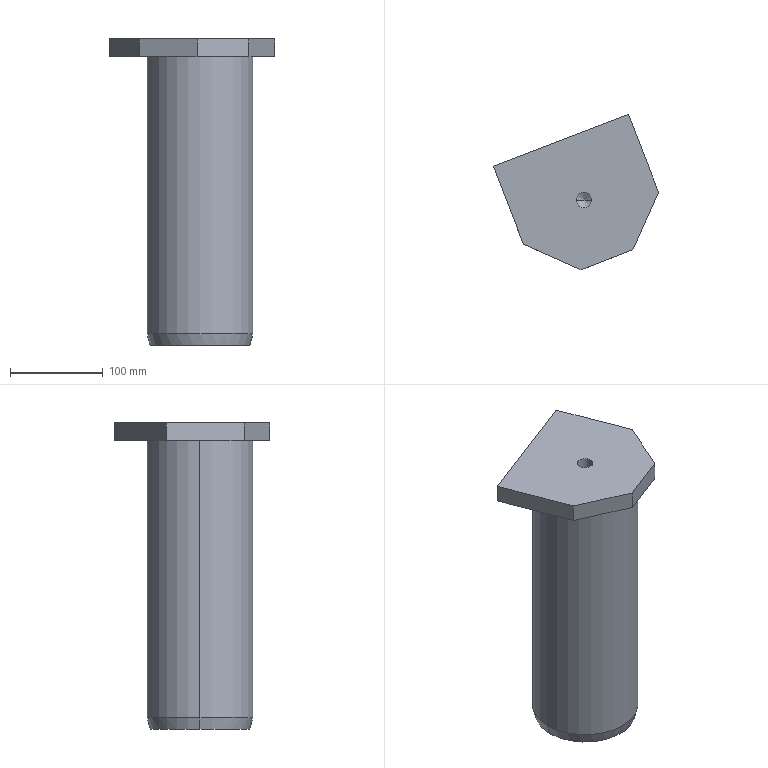Part | SolidWorks | features BaseBody 1, Scale 1 | 1 solid | 33 faces | box 177.912 x 167.575 x 330 mm | volume 3479602 mm3 | cylinder 12 | cone 12 | plane 9 | commonest cylinder face diameters 16.8 x10 114 x2
STEP:
#1=CARTESIAN_POINT('',(502.886,-738.285,240.227));
#2=VERTEX_POINT('',#1);
#3=CARTESIAN_POINT('',(616.886,-738.285,240.227));
#4=VERTEX_POINT('',#3);
#5=CARTESIAN_POINT('',(559.886,-738.285,240.227));
#6=DIRECTION('',(0.000000124,0.,-1.));
#7=DIRECTION('',(-1.,0.,-0.000000124));
#8=AXIS2_PLACEMENT_3D('',#5,#6,#7);
#9=CIRCLE('',#8,57.);
#10=EDGE_CURVE('',#2,#4,#9,.T.);
#11=ORIENTED_EDGE('',*,*,#10,.T.);
#12=CARTESIAN_POINT('',(616.886,-738.285,-58.573));
#13=VERTEX_POINT('',#12);
#14=CARTESIAN_POINT('',(616.886,-738.285,259.427));
#15=DIRECTION('',(0.000000124,0.,-1.));
#16=VECTOR('',#15,1000.);
#17=LINE('',#14,#16);
#18=EDGE_CURVE('',#4,#13,#17,.T.);
#19=ORIENTED_EDGE('',*,*,#18,.T.);
#20=CARTESIAN_POINT('',(502.886,-738.285,-58.573));
#21=VERTEX_POINT('',#20);
#22=CARTESIAN_POINT('',(559.886,-738.285,-58.573));
#23=DIRECTION('',(-0.000000124,0.,1.));
#24=DIRECTION('',(-1.,0.,-0.000000124));
#25=AXIS2_PLACEMENT_3D('',#22,#23,#24);
#26=CIRCLE('',#25,57.);
#27=EDGE_CURVE('',#13,#21,#26,.T.);
#28=ORIENTED_EDGE('',*,*,#27,.T.);
#29=CARTESIAN_POINT('',(502.886,-738.285,259.427));
#30=DIRECTION('',(0.000000124,0.,-1.));
#31=VECTOR('',#30,1000.);
#32=LINE('',#29,#31);
#33=EDGE_CURVE('',#2,#21,#32,.T.);
#34=ORIENTED_EDGE('',*,*,#33,.F.);
#35=EDGE_LOOP('',(#11,#19,#28,#34));
#36=FACE_OUTER_BOUND('',#35,.T.);
#37=CARTESIAN_POINT('',(559.886,-738.285,259.427));
#38=DIRECTION('',(0.000000124,0.,-1.));
#39=DIRECTION('',(-1.,0.,-0.000000124));
#40=AXIS2_PLACEMENT_3D('',#37,#38,#39);
#41=CYLINDRICAL_SURFACE('',#40,57.);
#42=ADVANCED_FACE('',(#36),#41,.T.);
#43=CARTESIAN_POINT('',(613.67,-738.285,-70.573));
#44=VERTEX_POINT('',#43);
#45=CARTESIAN_POINT('',(506.101,-738.285,-70.573));
#46=VERTEX_POINT('',#45);
#47=CARTESIAN_POINT('',(559.886,-738.285,-70.573));
#48=DIRECTION('',(-0.000000124,0.,1.));
#49=DIRECTION('',(1.,0.,0.000000124));
#50=AXIS2_PLACEMENT_3D('',#47,#48,#49);
#51=CIRCLE('',#50,53.785);
#52=EDGE_CURVE('',#44,#46,#51,.T.);
#53=ORIENTED_EDGE('',*,*,#52,.T.);
#54=CARTESIAN_POINT('',(502.886,-738.285,-58.573));
#55=DIRECTION('',(-0.2588,0.,0.9659));
#56=VECTOR('',#55,1000.);
#57=LINE('',#54,#56);
#58=EDGE_CURVE('',#46,#21,#57,.T.);
#59=ORIENTED_EDGE('',*,*,#58,.T.);
#60=ORIENTED_EDGE('',*,*,#27,.F.);
#61=CARTESIAN_POINT('',(616.886,-738.285,-58.573));
#62=DIRECTION('',(0.2588,0.,0.9659));
#63=VECTOR('',#62,1000.);
#64=LINE('',#61,#63);
#65=EDGE_CURVE('',#44,#13,#64,.T.);
#66=ORIENTED_EDGE('',*,*,#65,.F.);
#67=EDGE_LOOP('',(#53,#59,#60,#66));
#68=FACE_OUTER_BOUND('',#67,.T.);
#69=CARTESIAN_POINT('',(559.886,-738.285,-58.573));
#70=DIRECTION('',(-0.000000124,0.,1.));
#71=DIRECTION('',(1.,0.,0.000000124));
#72=AXIS2_PLACEMENT_3D('',#69,#70,#71);
#73=CONICAL_SURFACE('',#72,57.,0.2618);
#74=ADVANCED_FACE('',(#68),#73,.T.);
#75=CARTESIAN_POINT('',(535.388,-723.666,-70.573));
#76=VERTEX_POINT('',#75);
#77=CARTESIAN_POINT('',(518.588,-723.666,-70.573));
#78=VERTEX_POINT('',#77);
#79=CARTESIAN_POINT('',(526.988,-723.666,-70.573));
#80=DIRECTION('',(0.000000124,0.,-1.));
#81=DIRECTION('',(1.,0.,0.000000124));
#82=AXIS2_PLACEMENT_3D('',#79,#80,#81);
#83=CIRCLE('',#82,8.4);
#84=EDGE_CURVE('',#76,#78,#83,.T.);
#85=ORIENTED_EDGE('',*,*,#84,.T.);
#86=CARTESIAN_POINT('',(518.588,-723.666,-21.373));
#87=VERTEX_POINT('',#86);
#88=CARTESIAN_POINT('',(518.588,-723.666,-70.573));
#89=DIRECTION('',(-0.000000124,0.,1.));
#90=VECTOR('',#89,1000.);
#91=LINE('',#88,#90);
#92=EDGE_CURVE('',#78,#87,#91,.T.);
#93=ORIENTED_EDGE('',*,*,#92,.T.);
#94=CARTESIAN_POINT('',(535.388,-723.666,-21.373));
#95=VERTEX_POINT('',#94);
#96=CARTESIAN_POINT('',(526.988,-723.666,-21.373));
#97=DIRECTION('',(0.000000124,0.,-1.));
#98=DIRECTION('',(1.,0.,0.000000124));
#99=AXIS2_PLACEMENT_3D('',#96,#97,#98);
#100=CIRCLE('',#99,8.4);
#101=EDGE_CURVE('',#95,#87,#100,.T.);
#102=ORIENTED_EDGE('',*,*,#101,.F.);
#103=CARTESIAN_POINT('',(535.388,-723.666,-70.573));
#104=DIRECTION('',(-0.000000124,0.,1.));
#105=VECTOR('',#104,1000.);
#106=LINE('',#103,#105);
#107=EDGE_CURVE('',#76,#95,#106,.T.);
#108=ORIENTED_EDGE('',*,*,#107,.F.);
#109=EDGE_LOOP('',(#85,#93,#102,#108));
#110=FACE_OUTER_BOUND('',#109,.T.);
#111=CARTESIAN_POINT('',(526.988,-723.666,-70.573));
#112=DIRECTION('',(-0.000000124,0.,1.));
#113=DIRECTION('',(1.,0.,0.000000124));
#114=AXIS2_PLACEMENT_3D('',#111,#112,#113);
#115=CYLINDRICAL_SURFACE('',#114,8.4);
#116=ADVANCED_FACE('',(#110),#115,.F.);
#117=CARTESIAN_POINT('',(582.905,-705.387,-70.573));
#118=VERTEX_POINT('',#117);
#119=CARTESIAN_POINT('',(566.105,-705.387,-70.573));
#120=VERTEX_POINT('',#119);
#121=CARTESIAN_POINT('',(574.505,-705.387,-70.573));
#122=DIRECTION('',(0.000000124,0.,-1.));
#123=DIRECTION('',(1.,0.,0.000000124));
#124=AXIS2_PLACEMENT_3D('',#121,#122,#123);
#125=CIRCLE('',#124,8.4);
#126=EDGE_CURVE('',#118,#120,#125,.T.);
#127=ORIENTED_EDGE('',*,*,#126,.T.);
#128=CARTESIAN_POINT('',(566.105,-705.387,-21.373));
#129=VERTEX_POINT('',#128);
#130=CARTESIAN_POINT('',(566.105,-705.387,-70.573));
#131=DIRECTION('',(-0.000000124,0.,1.));
#132=VECTOR('',#131,1000.);
#133=LINE('',#130,#132);
#134=EDGE_CURVE('',#120,#129,#133,.T.);
#135=ORIENTED_EDGE('',*,*,#134,.T.);
#136=CARTESIAN_POINT('',(582.905,-705.387,-21.373));
#137=VERTEX_POINT('',#136);
#138=CARTESIAN_POINT('',(574.505,-705.387,-21.373));
#139=DIRECTION('',(0.000000124,0.,-1.));
#140=DIRECTION('',(1.,0.,0.000000124));
#141=AXIS2_PLACEMENT_3D('',#138,#139,#140);
#142=CIRCLE('',#141,8.4);
#143=EDGE_CURVE('',#137,#129,#142,.T.);
#144=ORIENTED_EDGE('',*,*,#143,.F.);
#145=CARTESIAN_POINT('',(582.905,-705.387,-70.573));
#146=DIRECTION('',(-0.000000124,0.,1.));
#147=VECTOR('',#146,1000.);
#148=LINE('',#145,#147);
#149=EDGE_CURVE('',#118,#137,#148,.T.);
#150=ORIENTED_EDGE('',*,*,#149,.F.);
#151=EDGE_LOOP('',(#127,#135,#144,#150));
#152=FACE_OUTER_BOUND('',#151,.T.);
#153=CARTESIAN_POINT('',(574.505,-705.387,-70.573));
#154=DIRECTION('',(-0.000000124,0.,1.));
#155=DIRECTION('',(1.,0.,0.000000124));
#156=AXIS2_PLACEMENT_3D('',#153,#154,#155);
#157=CYLINDRICAL_SURFACE('',#156,8.4);
#158=ADVANCED_FACE('',(#152),#157,.F.);
#159=CARTESIAN_POINT('',(601.184,-752.904,-70.573));
#160=VERTEX_POINT('',#159);
#161=CARTESIAN_POINT('',(584.384,-752.904,-70.573));
#162=VERTEX_POINT('',#161);
#163=CARTESIAN_POINT('',(592.784,-752.904,-70.573));
#164=DIRECTION('',(0.000000124,0.,-1.));
#165=DIRECTION('',(1.,0.,0.000000124));
#166=AXIS2_PLACEMENT_3D('',#163,#164,#165);
#167=CIRCLE('',#166,8.4);
#168=EDGE_CURVE('',#160,#162,#167,.T.);
#169=ORIENTED_EDGE('',*,*,#168,.T.);
#170=CARTESIAN_POINT('',(584.384,-752.904,-21.373));
#171=VERTEX_POINT('',#170);
#172=CARTESIAN_POINT('',(584.384,-752.904,-70.573));
#173=DIRECTION('',(-0.000000124,0.,1.));
#174=VECTOR('',#173,1000.);
#175=LINE('',#172,#174);
#176=EDGE_CURVE('',#162,#171,#175,.T.);
#177=ORIENTED_EDGE('',*,*,#176,.T.);
#178=CARTESIAN_POINT('',(601.184,-752.904,-21.373));
#179=VERTEX_POINT('',#178);
#180=CARTESIAN_POINT('',(592.784,-752.904,-21.373));
#181=DIRECTION('',(0.000000124,0.,-1.));
#182=DIRECTION('',(1.,0.,0.000000124));
#183=AXIS2_PLACEMENT_3D('',#180,#181,#182);
#184=CIRCLE('',#183,8.4);
#185=EDGE_CURVE('',#179,#171,#184,.T.);
#186=ORIENTED_EDGE('',*,*,#185,.F.);
#187=CARTESIAN_POINT('',(601.184,-752.904,-70.573));
#188=DIRECTION('',(-0.000000124,0.,1.));
#189=VECTOR('',#188,1000.);
#190=LINE('',#187,#189);
#191=EDGE_CURVE('',#160,#179,#190,.T.);
#192=ORIENTED_EDGE('',*,*,#191,.F.);
#193=EDGE_LOOP('',(#169,#177,#186,#192));
#194=FACE_OUTER_BOUND('',#193,.T.);
#195=CARTESIAN_POINT('',(592.784,-752.904,-70.573));
#196=DIRECTION('',(-0.000000124,0.,1.));
#197=DIRECTION('',(1.,0.,0.000000124));
#198=AXIS2_PLACEMENT_3D('',#195,#196,#197);
#199=CYLINDRICAL_SURFACE('',#198,8.4);
#200=ADVANCED_FACE('',(#194),#199,.F.);
#201=CARTESIAN_POINT('',(553.667,-771.183,-70.573));
#202=VERTEX_POINT('',#201);
#203=CARTESIAN_POINT('',(536.867,-771.183,-70.573));
#204=VERTEX_POINT('',#203);
#205=CARTESIAN_POINT('',(545.267,-771.183,-70.573));
#206=DIRECTION('',(0.000000124,0.,-1.));
#207=DIRECTION('',(1.,0.,0.000000124));
#208=AXIS2_PLACEMENT_3D('',#205,#206,#207);
#209=CIRCLE('',#208,8.4);
#210=EDGE_CURVE('',#202,#204,#209,.T.);
#211=ORIENTED_EDGE('',*,*,#210,.T.);
#212=CARTESIAN_POINT('',(536.867,-771.183,-21.373));
#213=VERTEX_POINT('',#212);
#214=CARTESIAN_POINT('',(536.867,-771.183,-70.573));
#215=DIRECTION('',(-0.000000124,0.,1.));
#216=VECTOR('',#215,1000.);
#217=LINE('',#214,#216);
#218=EDGE_CURVE('',#204,#213,#217,.T.);
#219=ORIENTED_EDGE('',*,*,#218,.T.);
#220=CARTESIAN_POINT('',(553.667,-771.183,-21.373));
#221=VERTEX_POINT('',#220);
#222=CARTESIAN_POINT('',(545.267,-771.183,-21.373));
#223=DIRECTION('',(0.000000124,0.,-1.));
#224=DIRECTION('',(1.,0.,0.000000124));
#225=AXIS2_PLACEMENT_3D('',#222,#223,#224);
#226=CIRCLE('',#225,8.4);
#227=EDGE_CURVE('',#221,#213,#226,.T.);
#228=ORIENTED_EDGE('',*,*,#227,.F.);
#229=CARTESIAN_POINT('',(553.667,-771.183,-70.573));
#230=DIRECTION('',(-0.000000124,0.,1.));
#231=VECTOR('',#230,1000.);
#232=LINE('',#229,#231);
#233=EDGE_CURVE('',#202,#221,#232,.T.);
#234=ORIENTED_EDGE('',*,*,#233,.F.);
#235=EDGE_LOOP('',(#211,#219,#228,#234));
#236=FACE_OUTER_BOUND('',#235,.T.);
#237=CARTESIAN_POINT('',(545.267,-771.183,-70.573));
#238=DIRECTION('',(-0.000000124,0.,1.));
#239=DIRECTION('',(1.,0.,0.000000124));
#240=AXIS2_PLACEMENT_3D('',#237,#238,#239);
#241=CYLINDRICAL_SURFACE('',#240,8.4);
#242=ADVANCED_FACE('',(#236),#241,.F.);
#243=CARTESIAN_POINT('',(526.988,-723.666,-16.326));
#244=VERTEX_POINT('',#243);
#245=CARTESIAN_POINT('',(518.588,-723.666,-21.373));
#246=DIRECTION('',(-0.8572,0.,-0.515));
#247=VECTOR('',#246,1000.);
#248=LINE('',#245,#247);
#249=EDGE_CURVE('',#244,#87,#248,.T.);
#250=ORIENTED_EDGE('',*,*,#249,.F.);
#251=CARTESIAN_POINT('',(535.388,-723.666,-21.373));
#252=DIRECTION('',(0.8572,0.,-0.515));
#253=VECTOR('',#252,1000.);
#254=LINE('',#251,#253);
#255=EDGE_CURVE('',#244,#95,#254,.T.);
#256=ORIENTED_EDGE('',*,*,#255,.T.);
#257=ORIENTED_EDGE('',*,*,#101,.T.);
#258=EDGE_LOOP('',(#250,#256,#257));
#259=FACE_OUTER_BOUND('',#258,.T.);
#260=CARTESIAN_POINT('',(526.988,-723.666,-21.373));
#261=DIRECTION('',(0.000000124,0.,-1.));
#262=DIRECTION('',(-1.,0.,-0.000000124));
#263=AXIS2_PLACEMENT_3D('',#260,#261,#262);
#264=CONICAL_SURFACE('',#263,8.4,1.03);
#265=ADVANCED_FACE('',(#259),#264,.F.);
#266=CARTESIAN_POINT('',(574.505,-705.387,-16.326));
#267=VERTEX_POINT('',#266);
#268=CARTESIAN_POINT('',(566.105,-705.387,-21.373));
#269=DIRECTION('',(-0.8572,0.,-0.515));
#270=VECTOR('',#269,1000.);
#271=LINE('',#268,#270);
#272=EDGE_CURVE('',#267,#129,#271,.T.);
#273=ORIENTED_EDGE('',*,*,#272,.F.);
#274=CARTESIAN_POINT('',(582.905,-705.387,-21.373));
#275=DIRECTION('',(0.8572,0.,-0.515));
#276=VECTOR('',#275,1000.);
#277=LINE('',#274,#276);
#278=EDGE_CURVE('',#267,#137,#277,.T.);
#279=ORIENTED_EDGE('',*,*,#278,.T.);
#280=ORIENTED_EDGE('',*,*,#143,.T.);
#281=EDGE_LOOP('',(#273,#279,#280));
#282=FACE_OUTER_BOUND('',#281,.T.);
#283=CARTESIAN_POINT('',(574.505,-705.387,-21.373));
#284=DIRECTION('',(0.000000124,0.,-1.));
#285=DIRECTION('',(-1.,0.,-0.000000124));
#286=AXIS2_PLACEMENT_3D('',#283,#284,#285);
#287=CONICAL_SURFACE('',#286,8.4,1.03);
#288=ADVANCED_FACE('',(#282),#287,.F.);
#289=CARTESIAN_POINT('',(592.784,-752.904,-16.326));
#290=VERTEX_POINT('',#289);
#291=CARTESIAN_POINT('',(584.384,-752.904,-21.373));
#292=DIRECTION('',(-0.8572,0.,-0.515));
#293=VECTOR('',#292,1000.);
#294=LINE('',#291,#293);
#295=EDGE_CURVE('',#290,#171,#294,.T.);
#296=ORIENTED_EDGE('',*,*,#295,.F.);
#297=CARTESIAN_POINT('',(601.184,-752.904,-21.373));
#298=DIRECTION('',(0.8572,0.,-0.515));
#299=VECTOR('',#298,1000.);
#300=LINE('',#297,#299);
#301=EDGE_CURVE('',#290,#179,#300,.T.);
#302=ORIENTED_EDGE('',*,*,#301,.T.);
#303=ORIENTED_EDGE('',*,*,#185,.T.);
#304=EDGE_LOOP('',(#296,#302,#303));
#305=FACE_OUTER_BOUND('',#304,.T.);
#306=CARTESIAN_POINT('',(592.784,-752.904,-21.373));
#307=DIRECTION('',(0.000000124,0.,-1.));
#308=DIRECTION('',(-1.,0.,-0.000000124));
#309=AXIS2_PLACEMENT_3D('',#306,#307,#308);
#310=CONICAL_SURFACE('',#309,8.4,1.03);
#311=ADVANCED_FACE('',(#305),#310,.F.);
#312=CARTESIAN_POINT('',(545.267,-771.183,-16.326));
#313=VERTEX_POINT('',#312);
#314=CARTESIAN_POINT('',(536.867,-771.183,-21.373));
#315=DIRECTION('',(-0.8572,0.,-0.515));
#316=VECTOR('',#315,1000.);
#317=LINE('',#314,#316);
#318=EDGE_CURVE('',#313,#213,#317,.T.);
#319=ORIENTED_EDGE('',*,*,#318,.F.);
#320=CARTESIAN_POINT('',(553.667,-771.183,-21.373));
#321=DIRECTION('',(0.8572,0.,-0.515));
#322=VECTOR('',#321,1000.);
#323=LINE('',#320,#322);
#324=EDGE_CURVE('',#313,#221,#323,.T.);
#325=ORIENTED_EDGE('',*,*,#324,.T.);
#326=ORIENTED_EDGE('',*,*,#227,.T.);
#327=EDGE_LOOP('',(#319,#325,#326));
#328=FACE_OUTER_BOUND('',#327,.T.);
#329=CARTESIAN_POINT('',(545.267,-771.183,-21.373));
#330=DIRECTION('',(0.000000124,0.,-1.));
#331=DIRECTION('',(-1.,0.,-0.000000124));
#332=AXIS2_PLACEMENT_3D('',#329,#330,#331);
#333=CONICAL_SURFACE('',#332,8.4,1.03);
#334=ADVANCED_FACE('',(#328),#333,.F.);
#335=CARTESIAN_POINT('',(568.286,-738.285,259.427));
#336=VERTEX_POINT('',#335);
#337=CARTESIAN_POINT('',(551.486,-738.285,259.427));
#338=VERTEX_POINT('',#337);
#339=CARTESIAN_POINT('',(559.886,-738.285,259.427));
#340=DIRECTION('',(0.000000124,0.,-1.));
#341=DIRECTION('',(-1.,0.,-0.000000124));
#342=AXIS2_PLACEMENT_3D('',#339,#340,#341);
#343=CIRCLE('',#342,8.4);
#344=EDGE_CURVE('',#336,#338,#343,.T.);
#345=ORIENTED_EDGE('',*,*,#344,.F.);
#346=CARTESIAN_POINT('',(568.286,-738.285,216.227));
#347=VERTEX_POINT('',#346);
#348=CARTESIAN_POINT('',(568.286,-738.285,259.427));
#349=DIRECTION('',(0.000000124,0.,-1.));
#350=VECTOR('',#349,1000.);
#351=LINE('',#348,#350);
#352=EDGE_CURVE('',#336,#347,#351,.T.);
#353=ORIENTED_EDGE('',*,*,#352,.T.);
#354=CARTESIAN_POINT('',(551.486,-738.285,216.227));
#355=VERTEX_POINT('',#354);
#356=CARTESIAN_POINT('',(559.886,-738.285,216.227));
#357=DIRECTION('',(-0.000000124,0.,1.));
#358=DIRECTION('',(-1.,0.,-0.000000124));
#359=AXIS2_PLACEMENT_3D('',#356,#357,#358);
#360=CIRCLE('',#359,8.4);
#361=EDGE_CURVE('',#355,#347,#360,.T.);
#362=ORIENTED_EDGE('',*,*,#361,.F.);
#363=CARTESIAN_POINT('',(551.486,-738.285,259.427));
#364=DIRECTION('',(0.000000124,0.,-1.));
#365=VECTOR('',#364,1000.);
#366=LINE('',#363,#365);
#367=EDGE_CURVE('',#338,#355,#366,.T.);
#368=ORIENTED_EDGE('',*,*,#367,.F.);
#369=EDGE_LOOP('',(#345,#353,#362,#368));
#370=FACE_OUTER_BOUND('',#369,.T.);
#371=CARTESIAN_POINT('',(559.886,-738.285,259.427));
#372=DIRECTION('',(0.000000124,0.,-1.));
#373=DIRECTION('',(-1.,0.,-0.000000124));
#374=AXIS2_PLACEMENT_3D('',#371,#372,#373);
#375=CYLINDRICAL_SURFACE('',#374,8.4);
#376=ADVANCED_FACE('',(#370),#375,.F.);
#377=CARTESIAN_POINT('',(559.886,-738.285,211.18));
#378=VERTEX_POINT('',#377);
#379=CARTESIAN_POINT('',(568.286,-738.285,216.227));
#380=DIRECTION('',(0.8572,0.,0.515));
#381=VECTOR('',#380,1000.);
#382=LINE('',#379,#381);
#383=EDGE_CURVE('',#378,#347,#382,.T.);
#384=ORIENTED_EDGE('',*,*,#383,.F.);
#385=CARTESIAN_POINT('',(551.486,-738.285,216.227));
#386=DIRECTION('',(-0.8572,0.,0.515));
#387=VECTOR('',#386,1000.);
#388=LINE('',#385,#387);
#389=EDGE_CURVE('',#378,#355,#388,.T.);
#390=ORIENTED_EDGE('',*,*,#389,.T.);
#391=ORIENTED_EDGE('',*,*,#361,.T.);
#392=EDGE_LOOP('',(#384,#390,#391));
#393=FACE_OUTER_BOUND('',#392,.T.);
#394=CARTESIAN_POINT('',(559.886,-738.285,216.227));
#395=DIRECTION('',(-0.000000124,0.,1.));
#396=DIRECTION('',(1.,0.,0.000000124));
#397=AXIS2_PLACEMENT_3D('',#394,#395,#396);
#398=CONICAL_SURFACE('',#397,8.4,1.03);
#399=ADVANCED_FACE('',(#393),#398,.F.);
#400=ORIENTED_EDGE('',*,*,#18,.F.);
#401=CARTESIAN_POINT('',(559.886,-738.285,240.227));
#402=DIRECTION('',(0.000000124,0.,-1.));
#403=DIRECTION('',(-1.,0.,-0.000000124));
#404=AXIS2_PLACEMENT_3D('',#401,#402,#403);
#405=CIRCLE('',#404,57.);
#406=EDGE_CURVE('',#4,#2,#405,.T.);
#407=ORIENTED_EDGE('',*,*,#406,.T.);
#408=ORIENTED_EDGE('',*,*,#33,.T.);
#409=CARTESIAN_POINT('',(559.886,-738.285,-58.573));
#410=DIRECTION('',(-0.000000124,0.,1.));
#411=DIRECTION('',(-1.,0.,-0.000000124));
#412=AXIS2_PLACEMENT_3D('',#409,#410,#411);
#413=CIRCLE('',#412,57.);
#414=EDGE_CURVE('',#21,#13,#413,.T.);
#415=ORIENTED_EDGE('',*,*,#414,.T.);
#416=EDGE_LOOP('',(#400,#407,#408,#415));
#417=FACE_OUTER_BOUND('',#416,.T.);
#418=CARTESIAN_POINT('',(559.886,-738.285,259.427));
#419=DIRECTION('',(0.000000124,0.,-1.));
#420=DIRECTION('',(-1.,0.,-0.000000124));
#421=AXIS2_PLACEMENT_3D('',#418,#419,#420);
#422=CYLINDRICAL_SURFACE('',#421,57.);
#423=ADVANCED_FACE('',(#417),#422,.T.);
#424=ORIENTED_EDGE('',*,*,#58,.F.);
#425=CARTESIAN_POINT('',(559.886,-738.285,-70.573));
#426=DIRECTION('',(-0.000000124,0.,1.));
#427=DIRECTION('',(1.,0.,0.000000124));
#428=AXIS2_PLACEMENT_3D('',#425,#426,#427);
#429=CIRCLE('',#428,53.785);
#430=EDGE_CURVE('',#46,#44,#429,.T.);
#431=ORIENTED_EDGE('',*,*,#430,.T.);
#432=ORIENTED_EDGE('',*,*,#65,.T.);
#433=ORIENTED_EDGE('',*,*,#414,.F.);
#434=EDGE_LOOP('',(#424,#431,#432,#433));
#435=FACE_OUTER_BOUND('',#434,.T.);
#436=CARTESIAN_POINT('',(559.886,-738.285,-58.573));
#437=DIRECTION('',(-0.000000124,0.,1.));
#438=DIRECTION('',(1.,0.,0.000000124));
#439=AXIS2_PLACEMENT_3D('',#436,#437,#438);
#440=CONICAL_SURFACE('',#439,57.,0.2618);
#441=ADVANCED_FACE('',(#435),#440,.T.);
#442=CARTESIAN_POINT('',(640.225,-729.879,240.227));
#443=VERTEX_POINT('',#442);
#444=CARTESIAN_POINT('',(607.911,-645.88,240.227));
#445=VERTEX_POINT('',#444);
#446=CARTESIAN_POINT('',(640.225,-729.879,240.227));
#447=DIRECTION('',(-0.359,0.9333,-0.000000044));
#448=VECTOR('',#447,1000.);
#449=LINE('',#446,#448);
#450=EDGE_CURVE('',#443,#445,#449,.T.);
#451=ORIENTED_EDGE('',*,*,#450,.F.);
#452=CARTESIAN_POINT('',(612.659,-791.913,240.227));
#453=VERTEX_POINT('',#452);
#454=CARTESIAN_POINT('',(612.659,-791.913,240.227));
#455=DIRECTION('',(0.4061,0.9138,0.00000005));
#456=VECTOR('',#455,1000.);
#457=LINE('',#454,#456);
#458=EDGE_CURVE('',#453,#443,#457,.T.);
#459=ORIENTED_EDGE('',*,*,#458,.F.);
#460=CARTESIAN_POINT('',(556.66,-813.455,240.227));
#461=VERTEX_POINT('',#460);
#462=CARTESIAN_POINT('',(612.659,-791.913,240.227));
#463=DIRECTION('',(0.9333,0.359,0.000000116));
#464=VECTOR('',#463,1000.);
#465=LINE('',#462,#464);
#466=EDGE_CURVE('',#461,#453,#465,.T.);
#467=ORIENTED_EDGE('',*,*,#466,.F.);
#468=CARTESIAN_POINT('',(494.627,-785.89,240.227));
#469=VERTEX_POINT('',#468);
#470=CARTESIAN_POINT('',(556.66,-813.455,240.227));
#471=DIRECTION('',(0.9138,-0.4061,0.000000113));
#472=VECTOR('',#471,1000.);
#473=LINE('',#470,#472);
#474=EDGE_CURVE('',#469,#461,#473,.T.);
#475=ORIENTED_EDGE('',*,*,#474,.F.);
#476=CARTESIAN_POINT('',(462.313,-701.891,240.227));
#477=VERTEX_POINT('',#476);
#478=CARTESIAN_POINT('',(462.313,-701.891,240.227));
#479=DIRECTION('',(0.359,-0.9333,0.000000044));
#480=VECTOR('',#479,1000.);
#481=LINE('',#478,#480);
#482=EDGE_CURVE('',#477,#469,#481,.T.);
#483=ORIENTED_EDGE('',*,*,#482,.F.);
#484=CARTESIAN_POINT('',(607.911,-645.88,240.227));
#485=DIRECTION('',(-0.9333,-0.359,-0.000000116));
#486=VECTOR('',#485,1000.);
#487=LINE('',#484,#486);
#488=EDGE_CURVE('',#445,#477,#487,.T.);
#489=ORIENTED_EDGE('',*,*,#488,.F.);
#490=EDGE_LOOP('',(#451,#459,#467,#475,#483,#489));
#491=FACE_OUTER_BOUND('',#490,.T.);
#492=ORIENTED_EDGE('',*,*,#10,.F.);
#493=ORIENTED_EDGE('',*,*,#406,.F.);
#494=EDGE_LOOP('',(#492,#493));
#495=FACE_BOUND('',#494,.T.);
#496=CARTESIAN_POINT('',(-1469.793,3990.883,240.227));
#497=DIRECTION('',(-0.000000124,0.,1.));
#498=DIRECTION('',(1.,0.,0.000000124));
#499=AXIS2_PLACEMENT_3D('',#496,#497,#498);
#500=PLANE('',#499);
#501=ADVANCED_FACE('',(#491,#495),#500,.F.);
#502=ORIENTED_EDGE('',*,*,#52,.F.);
#503=ORIENTED_EDGE('',*,*,#430,.F.);
#504=EDGE_LOOP('',(#502,#503));
#505=FACE_OUTER_BOUND('',#504,.T.);
#506=ORIENTED_EDGE('',*,*,#84,.F.);
#507=CARTESIAN_POINT('',(526.988,-723.666,-70.573));
#508=DIRECTION('',(0.000000124,0.,-1.));
#509=DIRECTION('',(1.,0.,0.000000124));
#510=AXIS2_PLACEMENT_3D('',#507,#508,#509);
#511=CIRCLE('',#510,8.4);
#512=EDGE_CURVE('',#78,#76,#511,.T.);
#513=ORIENTED_EDGE('',*,*,#512,.F.);
#514=EDGE_LOOP('',(#506,#513));
#515=FACE_BOUND('',#514,.T.);
#516=ORIENTED_EDGE('',*,*,#126,.F.);
#517=CARTESIAN_POINT('',(574.505,-705.387,-70.573));
#518=DIRECTION('',(0.000000124,0.,-1.));
#519=DIRECTION('',(1.,0.,0.000000124));
#520=AXIS2_PLACEMENT_3D('',#517,#518,#519);
#521=CIRCLE('',#520,8.4);
#522=EDGE_CURVE('',#120,#118,#521,.T.);
#523=ORIENTED_EDGE('',*,*,#522,.F.);
#524=EDGE_LOOP('',(#516,#523));
#525=FACE_BOUND('',#524,.T.);
#526=ORIENTED_EDGE('',*,*,#168,.F.);
#527=CARTESIAN_POINT('',(592.784,-752.904,-70.573));
#528=DIRECTION('',(0.000000124,0.,-1.));
#529=DIRECTION('',(1.,0.,0.000000124));
#530=AXIS2_PLACEMENT_3D('',#527,#528,#529);
#531=CIRCLE('',#530,8.4);
#532=EDGE_CURVE('',#162,#160,#531,.T.);
#533=ORIENTED_EDGE('',*,*,#532,.F.);
#534=EDGE_LOOP('',(#526,#533));
#535=FACE_BOUND('',#534,.T.);
#536=ORIENTED_EDGE('',*,*,#210,.F.);
#537=CARTESIAN_POINT('',(545.267,-771.183,-70.573));
#538=DIRECTION('',(0.000000124,0.,-1.));
#539=DIRECTION('',(1.,0.,0.000000124));
#540=AXIS2_PLACEMENT_3D('',#537,#538,#539);
#541=CIRCLE('',#540,8.4);
#542=EDGE_CURVE('',#204,#202,#541,.T.);
#543=ORIENTED_EDGE('',*,*,#542,.F.);
#544=EDGE_LOOP('',(#536,#543));
#545=FACE_BOUND('',#544,.T.);
#546=CARTESIAN_POINT('',(579.197,-788.483,-70.573));
#547=DIRECTION('',(-0.000000124,0.,1.));
#548=DIRECTION('',(1.,0.,0.000000124));
#549=AXIS2_PLACEMENT_3D('',#546,#547,#548);
#550=PLANE('',#549);
#551=ADVANCED_FACE('',(#505,#515,#525,#535,#545),#550,.F.);
#552=CARTESIAN_POINT('',(607.911,-645.88,259.427));
#553=VERTEX_POINT('',#552);
#554=CARTESIAN_POINT('',(607.911,-645.88,259.427));
#555=DIRECTION('',(-0.000000016,0.000000042,1.));
#556=VECTOR('',#555,1000.);
#557=LINE('',#554,#556);
#558=EDGE_CURVE('',#445,#553,#557,.T.);
#559=ORIENTED_EDGE('',*,*,#558,.F.);
#560=ORIENTED_EDGE('',*,*,#488,.T.);
#561=CARTESIAN_POINT('',(462.313,-701.891,259.427));
#562=VERTEX_POINT('',#561);
#563=CARTESIAN_POINT('',(462.313,-701.891,259.427));
#564=DIRECTION('',(0.000000016,-0.000000042,-1.));
#565=VECTOR('',#564,1000.);
#566=LINE('',#563,#565);
#567=EDGE_CURVE('',#562,#477,#566,.T.);
#568=ORIENTED_EDGE('',*,*,#567,.F.);
#569=CARTESIAN_POINT('',(607.911,-645.88,259.427));
#570=DIRECTION('',(-0.9333,-0.359,-0.000000124));
#571=VECTOR('',#570,1000.);
#572=LINE('',#569,#571);
#573=EDGE_CURVE('',#553,#562,#572,.T.);
#574=ORIENTED_EDGE('',*,*,#573,.F.);
#575=EDGE_LOOP('',(#559,#560,#568,#574));
#576=FACE_OUTER_BOUND('',#575,.T.);
#577=CARTESIAN_POINT('',(607.911,-645.88,259.427));
#578=DIRECTION('',(0.359,-0.9333,0.000000044));
#579=DIRECTION('',(0.9333,0.359,0.));
#580=AXIS2_PLACEMENT_3D('',#577,#578,#579);
#581=PLANE('',#580);
#582=ADVANCED_FACE('',(#576),#581,.F.);
#583=CARTESIAN_POINT('',(640.225,-729.879,259.427));
#584=VERTEX_POINT('',#583);
#585=CARTESIAN_POINT('',(640.225,-729.879,259.427));
#586=DIRECTION('',(-0.000000108,-0.000000042,1.));
#587=VECTOR('',#586,1000.);
#588=LINE('',#585,#587);
#589=EDGE_CURVE('',#443,#584,#588,.T.);
#590=ORIENTED_EDGE('',*,*,#589,.F.);
#591=ORIENTED_EDGE('',*,*,#450,.T.);
#592=ORIENTED_EDGE('',*,*,#558,.T.);
#593=CARTESIAN_POINT('',(640.225,-729.879,259.427));
#594=DIRECTION('',(-0.359,0.9333,0.));
#595=VECTOR('',#594,1000.);
#596=LINE('',#593,#595);
#597=EDGE_CURVE('',#584,#553,#596,.T.);
#598=ORIENTED_EDGE('',*,*,#597,.F.);
#599=EDGE_LOOP('',(#590,#591,#592,#598));
#600=FACE_OUTER_BOUND('',#599,.T.);
#601=CARTESIAN_POINT('',(640.225,-729.879,259.427));
#602=DIRECTION('',(-0.9333,-0.359,-0.000000116));
#603=DIRECTION('',(0.359,-0.9333,0.));
#604=AXIS2_PLACEMENT_3D('',#601,#602,#603);
#605=PLANE('',#604);
#606=ADVANCED_FACE('',(#600),#605,.F.);
#607=CARTESIAN_POINT('',(612.659,-791.913,259.427));
#608=VERTEX_POINT('',#607);
#609=CARTESIAN_POINT('',(612.659,-791.913,259.427));
#610=DIRECTION('',(-0.000000124,0.,1.));
#611=VECTOR('',#610,1000.);
#612=LINE('',#609,#611);
#613=EDGE_CURVE('',#453,#608,#612,.T.);
#614=ORIENTED_EDGE('',*,*,#613,.F.);
#615=ORIENTED_EDGE('',*,*,#458,.T.);
#616=ORIENTED_EDGE('',*,*,#589,.T.);
#617=CARTESIAN_POINT('',(640.225,-729.879,259.427));
#618=DIRECTION('',(0.4061,0.9138,0.));
#619=VECTOR('',#618,1000.);
#620=LINE('',#617,#619);
#621=EDGE_CURVE('',#608,#584,#620,.T.);
#622=ORIENTED_EDGE('',*,*,#621,.F.);
#623=EDGE_LOOP('',(#614,#615,#616,#622));
#624=FACE_OUTER_BOUND('',#623,.T.);
#625=CARTESIAN_POINT('',(640.225,-729.879,259.427));
#626=DIRECTION('',(-0.9138,0.4061,-0.000000113));
#627=DIRECTION('',(-0.4061,-0.9138,0.));
#628=AXIS2_PLACEMENT_3D('',#625,#626,#627);
#629=PLANE('',#628);
#630=ADVANCED_FACE('',(#624),#629,.F.);
#631=CARTESIAN_POINT('',(556.66,-813.455,259.427));
#632=VERTEX_POINT('',#631);
#633=CARTESIAN_POINT('',(556.66,-813.455,259.427));
#634=DIRECTION('',(-0.000000124,0.,1.));
#635=VECTOR('',#634,1000.);
#636=LINE('',#633,#635);
#637=EDGE_CURVE('',#461,#632,#636,.T.);
#638=ORIENTED_EDGE('',*,*,#637,.F.);
#639=ORIENTED_EDGE('',*,*,#466,.T.);
#640=ORIENTED_EDGE('',*,*,#613,.T.);
#641=CARTESIAN_POINT('',(556.66,-813.455,259.427));
#642=DIRECTION('',(0.9333,0.359,0.000000116));
#643=VECTOR('',#642,1000.);
#644=LINE('',#641,#643);
#645=EDGE_CURVE('',#632,#608,#644,.T.);
#646=ORIENTED_EDGE('',*,*,#645,.F.);
#647=EDGE_LOOP('',(#638,#639,#640,#646));
#648=FACE_OUTER_BOUND('',#647,.T.);
#649=CARTESIAN_POINT('',(612.659,-791.913,259.427));
#650=DIRECTION('',(-0.359,0.9333,-0.000000044));
#651=DIRECTION('',(-0.9333,-0.359,0.));
#652=AXIS2_PLACEMENT_3D('',#649,#650,#651);
#653=PLANE('',#652);
#654=ADVANCED_FACE('',(#648),#653,.F.);
#655=CARTESIAN_POINT('',(494.627,-785.89,259.427));
#656=VERTEX_POINT('',#655);
#657=CARTESIAN_POINT('',(494.627,-785.89,259.427));
#658=DIRECTION('',(-0.000000108,-0.000000042,1.));
#659=VECTOR('',#658,1000.);
#660=LINE('',#657,#659);
#661=EDGE_CURVE('',#469,#656,#660,.T.);
#662=ORIENTED_EDGE('',*,*,#661,.F.);
#663=ORIENTED_EDGE('',*,*,#474,.T.);
#664=ORIENTED_EDGE('',*,*,#637,.T.);
#665=CARTESIAN_POINT('',(494.627,-785.89,259.427));
#666=DIRECTION('',(0.9138,-0.4061,0.000000113));
#667=VECTOR('',#666,1000.);
#668=LINE('',#665,#667);
#669=EDGE_CURVE('',#656,#632,#668,.T.);
#670=ORIENTED_EDGE('',*,*,#669,.F.);
#671=EDGE_LOOP('',(#662,#663,#664,#670));
#672=FACE_OUTER_BOUND('',#671,.T.);
#673=CARTESIAN_POINT('',(556.66,-813.455,259.427));
#674=DIRECTION('',(0.4061,0.9138,0.00000005));
#675=DIRECTION('',(-0.9138,0.4061,0.));
#676=AXIS2_PLACEMENT_3D('',#673,#674,#675);
#677=PLANE('',#676);
#678=ADVANCED_FACE('',(#672),#677,.F.);
#679=ORIENTED_EDGE('',*,*,#567,.T.);
#680=ORIENTED_EDGE('',*,*,#482,.T.);
#681=ORIENTED_EDGE('',*,*,#661,.T.);
#682=CARTESIAN_POINT('',(494.627,-785.89,259.427));
#683=DIRECTION('',(0.359,-0.9333,0.));
#684=VECTOR('',#683,1000.);
#685=LINE('',#682,#684);
#686=EDGE_CURVE('',#562,#656,#685,.T.);
#687=ORIENTED_EDGE('',*,*,#686,.F.);
#688=EDGE_LOOP('',(#679,#680,#681,#687));
#689=FACE_OUTER_BOUND('',#688,.T.);
#690=CARTESIAN_POINT('',(494.627,-785.89,259.427));
#691=DIRECTION('',(0.9333,0.359,0.000000116));
#692=DIRECTION('',(-0.359,0.9333,0.));
#693=AXIS2_PLACEMENT_3D('',#690,#691,#692);
#694=PLANE('',#693);
#695=ADVANCED_FACE('',(#689),#694,.F.);
#696=ORIENTED_EDGE('',*,*,#92,.F.);
#697=ORIENTED_EDGE('',*,*,#512,.T.);
#698=ORIENTED_EDGE('',*,*,#107,.T.);
#699=CARTESIAN_POINT('',(526.988,-723.666,-21.373));
#700=DIRECTION('',(0.000000124,0.,-1.));
#701=DIRECTION('',(1.,0.,0.000000124));
#702=AXIS2_PLACEMENT_3D('',#699,#700,#701);
#703=CIRCLE('',#702,8.4);
#704=EDGE_CURVE('',#87,#95,#703,.T.);
#705=ORIENTED_EDGE('',*,*,#704,.F.);
#706=EDGE_LOOP('',(#696,#697,#698,#705));
#707=FACE_OUTER_BOUND('',#706,.T.);
#708=CARTESIAN_POINT('',(526.988,-723.666,-70.573));
#709=DIRECTION('',(-0.000000124,0.,1.));
#710=DIRECTION('',(1.,0.,0.000000124));
#711=AXIS2_PLACEMENT_3D('',#708,#709,#710);
#712=CYLINDRICAL_SURFACE('',#711,8.4);
#713=ADVANCED_FACE('',(#707),#712,.F.);
#714=ORIENTED_EDGE('',*,*,#134,.F.);
#715=ORIENTED_EDGE('',*,*,#522,.T.);
#716=ORIENTED_EDGE('',*,*,#149,.T.);
#717=CARTESIAN_POINT('',(574.505,-705.387,-21.373));
#718=DIRECTION('',(0.000000124,0.,-1.));
#719=DIRECTION('',(1.,0.,0.000000124));
#720=AXIS2_PLACEMENT_3D('',#717,#718,#719);
#721=CIRCLE('',#720,8.4);
#722=EDGE_CURVE('',#129,#137,#721,.T.);
#723=ORIENTED_EDGE('',*,*,#722,.F.);
#724=EDGE_LOOP('',(#714,#715,#716,#723));
#725=FACE_OUTER_BOUND('',#724,.T.);
#726=CARTESIAN_POINT('',(574.505,-705.387,-70.573));
#727=DIRECTION('',(-0.000000124,0.,1.));
#728=DIRECTION('',(1.,0.,0.000000124));
#729=AXIS2_PLACEMENT_3D('',#726,#727,#728);
#730=CYLINDRICAL_SURFACE('',#729,8.4);
#731=ADVANCED_FACE('',(#725),#730,.F.);
#732=ORIENTED_EDGE('',*,*,#176,.F.);
#733=ORIENTED_EDGE('',*,*,#532,.T.);
#734=ORIENTED_EDGE('',*,*,#191,.T.);
#735=CARTESIAN_POINT('',(592.784,-752.904,-21.373));
#736=DIRECTION('',(0.000000124,0.,-1.));
#737=DIRECTION('',(1.,0.,0.000000124));
#738=AXIS2_PLACEMENT_3D('',#735,#736,#737);
#739=CIRCLE('',#738,8.4);
#740=EDGE_CURVE('',#171,#179,#739,.T.);
#741=ORIENTED_EDGE('',*,*,#740,.F.);
#742=EDGE_LOOP('',(#732,#733,#734,#741));
#743=FACE_OUTER_BOUND('',#742,.T.);
#744=CARTESIAN_POINT('',(592.784,-752.904,-70.573));
#745=DIRECTION('',(-0.000000124,0.,1.));
#746=DIRECTION('',(1.,0.,0.000000124));
#747=AXIS2_PLACEMENT_3D('',#744,#745,#746);
#748=CYLINDRICAL_SURFACE('',#747,8.4);
#749=ADVANCED_FACE('',(#743),#748,.F.);
#750=ORIENTED_EDGE('',*,*,#218,.F.);
#751=ORIENTED_EDGE('',*,*,#542,.T.);
#752=ORIENTED_EDGE('',*,*,#233,.T.);
#753=CARTESIAN_POINT('',(545.267,-771.183,-21.373));
#754=DIRECTION('',(0.000000124,0.,-1.));
#755=DIRECTION('',(1.,0.,0.000000124));
#756=AXIS2_PLACEMENT_3D('',#753,#754,#755);
#757=CIRCLE('',#756,8.4);
#758=EDGE_CURVE('',#213,#221,#757,.T.);
#759=ORIENTED_EDGE('',*,*,#758,.F.);
#760=EDGE_LOOP('',(#750,#751,#752,#759));
#761=FACE_OUTER_BOUND('',#760,.T.);
#762=CARTESIAN_POINT('',(545.267,-771.183,-70.573));
#763=DIRECTION('',(-0.000000124,0.,1.));
#764=DIRECTION('',(1.,0.,0.000000124));
#765=AXIS2_PLACEMENT_3D('',#762,#763,#764);
#766=CYLINDRICAL_SURFACE('',#765,8.4);
#767=ADVANCED_FACE('',(#761),#766,.F.);
#768=CARTESIAN_POINT('',(559.886,-738.285,259.427));
#769=DIRECTION('',(0.000000124,0.,-1.));
#770=DIRECTION('',(-1.,0.,-0.000000124));
#771=AXIS2_PLACEMENT_3D('',#768,#769,#770);
#772=CIRCLE('',#771,8.4);
#773=EDGE_CURVE('',#338,#336,#772,.T.);
#774=ORIENTED_EDGE('',*,*,#773,.T.);
#775=ORIENTED_EDGE('',*,*,#344,.T.);
#776=EDGE_LOOP('',(#774,#775));
#777=FACE_BOUND('',#776,.T.);
#778=ORIENTED_EDGE('',*,*,#669,.T.);
#779=ORIENTED_EDGE('',*,*,#645,.T.);
#780=ORIENTED_EDGE('',*,*,#621,.T.);
#781=ORIENTED_EDGE('',*,*,#597,.T.);
#782=ORIENTED_EDGE('',*,*,#573,.T.);
#783=ORIENTED_EDGE('',*,*,#686,.T.);
#784=EDGE_LOOP('',(#778,#779,#780,#781,#782,#783));
#785=FACE_OUTER_BOUND('',#784,.T.);
#786=CARTESIAN_POINT('',(-1469.793,3990.883,259.427));
#787=DIRECTION('',(-0.000000124,0.,1.));
#788=DIRECTION('',(1.,0.,0.000000124));
#789=AXIS2_PLACEMENT_3D('',#786,#787,#788);
#790=PLANE('',#789);
#791=ADVANCED_FACE('',(#777,#785),#790,.T.);
#792=ORIENTED_EDGE('',*,*,#255,.F.);
#793=ORIENTED_EDGE('',*,*,#249,.T.);
#794=ORIENTED_EDGE('',*,*,#704,.T.);
#795=EDGE_LOOP('',(#792,#793,#794));
#796=FACE_OUTER_BOUND('',#795,.T.);
#797=CARTESIAN_POINT('',(526.988,-723.666,-21.373));
#798=DIRECTION('',(0.000000124,0.,-1.));
#799=DIRECTION('',(-1.,0.,-0.000000124));
#800=AXIS2_PLACEMENT_3D('',#797,#798,#799);
#801=CONICAL_SURFACE('',#800,8.4,1.03);
#802=ADVANCED_FACE('',(#796),#801,.F.);
#803=ORIENTED_EDGE('',*,*,#278,.F.);
#804=ORIENTED_EDGE('',*,*,#272,.T.);
#805=ORIENTED_EDGE('',*,*,#722,.T.);
#806=EDGE_LOOP('',(#803,#804,#805));
#807=FACE_OUTER_BOUND('',#806,.T.);
#808=CARTESIAN_POINT('',(574.505,-705.387,-21.373));
#809=DIRECTION('',(0.000000124,0.,-1.));
#810=DIRECTION('',(-1.,0.,-0.000000124));
#811=AXIS2_PLACEMENT_3D('',#808,#809,#810);
#812=CONICAL_SURFACE('',#811,8.4,1.03);
#813=ADVANCED_FACE('',(#807),#812,.F.);
#814=ORIENTED_EDGE('',*,*,#301,.F.);
#815=ORIENTED_EDGE('',*,*,#295,.T.);
#816=ORIENTED_EDGE('',*,*,#740,.T.);
#817=EDGE_LOOP('',(#814,#815,#816));
#818=FACE_OUTER_BOUND('',#817,.T.);
#819=CARTESIAN_POINT('',(592.784,-752.904,-21.373));
#820=DIRECTION('',(0.000000124,0.,-1.));
#821=DIRECTION('',(-1.,0.,-0.000000124));
#822=AXIS2_PLACEMENT_3D('',#819,#820,#821);
#823=CONICAL_SURFACE('',#822,8.4,1.03);
#824=ADVANCED_FACE('',(#818),#823,.F.);
#825=ORIENTED_EDGE('',*,*,#324,.F.);
#826=ORIENTED_EDGE('',*,*,#318,.T.);
#827=ORIENTED_EDGE('',*,*,#758,.T.);
#828=EDGE_LOOP('',(#825,#826,#827));
#829=FACE_OUTER_BOUND('',#828,.T.);
#830=CARTESIAN_POINT('',(545.267,-771.183,-21.373));
#831=DIRECTION('',(0.000000124,0.,-1.));
#832=DIRECTION('',(-1.,0.,-0.000000124));
#833=AXIS2_PLACEMENT_3D('',#830,#831,#832);
#834=CONICAL_SURFACE('',#833,8.4,1.03);
#835=ADVANCED_FACE('',(#829),#834,.F.);
#836=ORIENTED_EDGE('',*,*,#352,.F.);
#837=ORIENTED_EDGE('',*,*,#773,.F.);
#838=ORIENTED_EDGE('',*,*,#367,.T.);
#839=CARTESIAN_POINT('',(559.886,-738.285,216.227));
#840=DIRECTION('',(-0.000000124,0.,1.));
#841=DIRECTION('',(-1.,0.,-0.000000124));
#842=AXIS2_PLACEMENT_3D('',#839,#840,#841);
#843=CIRCLE('',#842,8.4);
#844=EDGE_CURVE('',#347,#355,#843,.T.);
#845=ORIENTED_EDGE('',*,*,#844,.F.);
#846=EDGE_LOOP('',(#836,#837,#838,#845));
#847=FACE_OUTER_BOUND('',#846,.T.);
#848=CARTESIAN_POINT('',(559.886,-738.285,259.427));
#849=DIRECTION('',(0.000000124,0.,-1.));
#850=DIRECTION('',(-1.,0.,-0.000000124));
#851=AXIS2_PLACEMENT_3D('',#848,#849,#850);
#852=CYLINDRICAL_SURFACE('',#851,8.4);
#853=ADVANCED_FACE('',(#847),#852,.F.);
#854=ORIENTED_EDGE('',*,*,#389,.F.);
#855=ORIENTED_EDGE('',*,*,#383,.T.);
#856=ORIENTED_EDGE('',*,*,#844,.T.);
#857=EDGE_LOOP('',(#854,#855,#856));
#858=FACE_OUTER_BOUND('',#857,.T.);
#859=CARTESIAN_POINT('',(559.886,-738.285,216.227));
#860=DIRECTION('',(-0.000000124,0.,1.));
#861=DIRECTION('',(1.,0.,0.000000124));
#862=AXIS2_PLACEMENT_3D('',#859,#860,#861);
#863=CONICAL_SURFACE('',#862,8.4,1.03);
#864=ADVANCED_FACE('',(#858),#863,.F.);
#865=CLOSED_SHELL('',(#42,#74,#116,#158,#200,#242,#265,#288,#311,#334,#376,#399,#423,#441,#501,#551,#582,#606,#630,#654,#678,#695,#713,#731,#749,#767,#791,#802,#813,#824,#835,#853,#864));
#866=MANIFOLD_SOLID_BREP('',#865);
#867=CARTESIAN_POINT('',(0.,0.,0.));
#868=DIRECTION('',(0.,0.,1.));
#869=DIRECTION('',(1.,0.,0.));
#870=AXIS2_PLACEMENT_3D('',#867,#868,#869);
#871=(LENGTH_UNIT()NAMED_UNIT(*)SI_UNIT(.MILLI.,.METRE.));
#872=UNCERTAINTY_MEASURE_WITH_UNIT(LENGTH_MEASURE(0.00001),#871,'','');
#873=(NAMED_UNIT(*)PLANE_ANGLE_UNIT()SI_UNIT($,.RADIAN.));
#874=(NAMED_UNIT(*)SI_UNIT($,.STERADIAN.)SOLID_ANGLE_UNIT());
#875=(GEOMETRIC_REPRESENTATION_CONTEXT(3)GLOBAL_UNCERTAINTY_ASSIGNED_CONTEXT((#872))GLOBAL_UNIT_ASSIGNED_CONTEXT((#871,#873,#874))REPRESENTATION_CONTEXT('',''));
#876=ADVANCED_BREP_SHAPE_REPRESENTATION('',(#866,#870),#875);